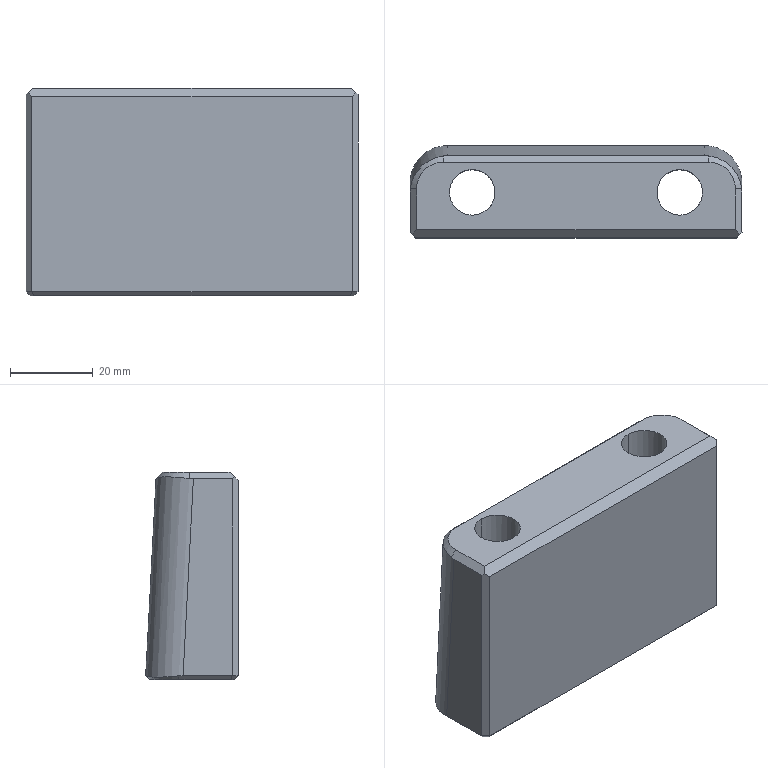Part | Creo | 1 solid | 41 faces | box 80 x 22.321 x 50 mm | volume 68055 mm3 | plane 21 | cylinder 14 | spline 4 | cone 2 | commonest cylinder face diameters 18 x6 11 x4 6.8 x2 8 x2